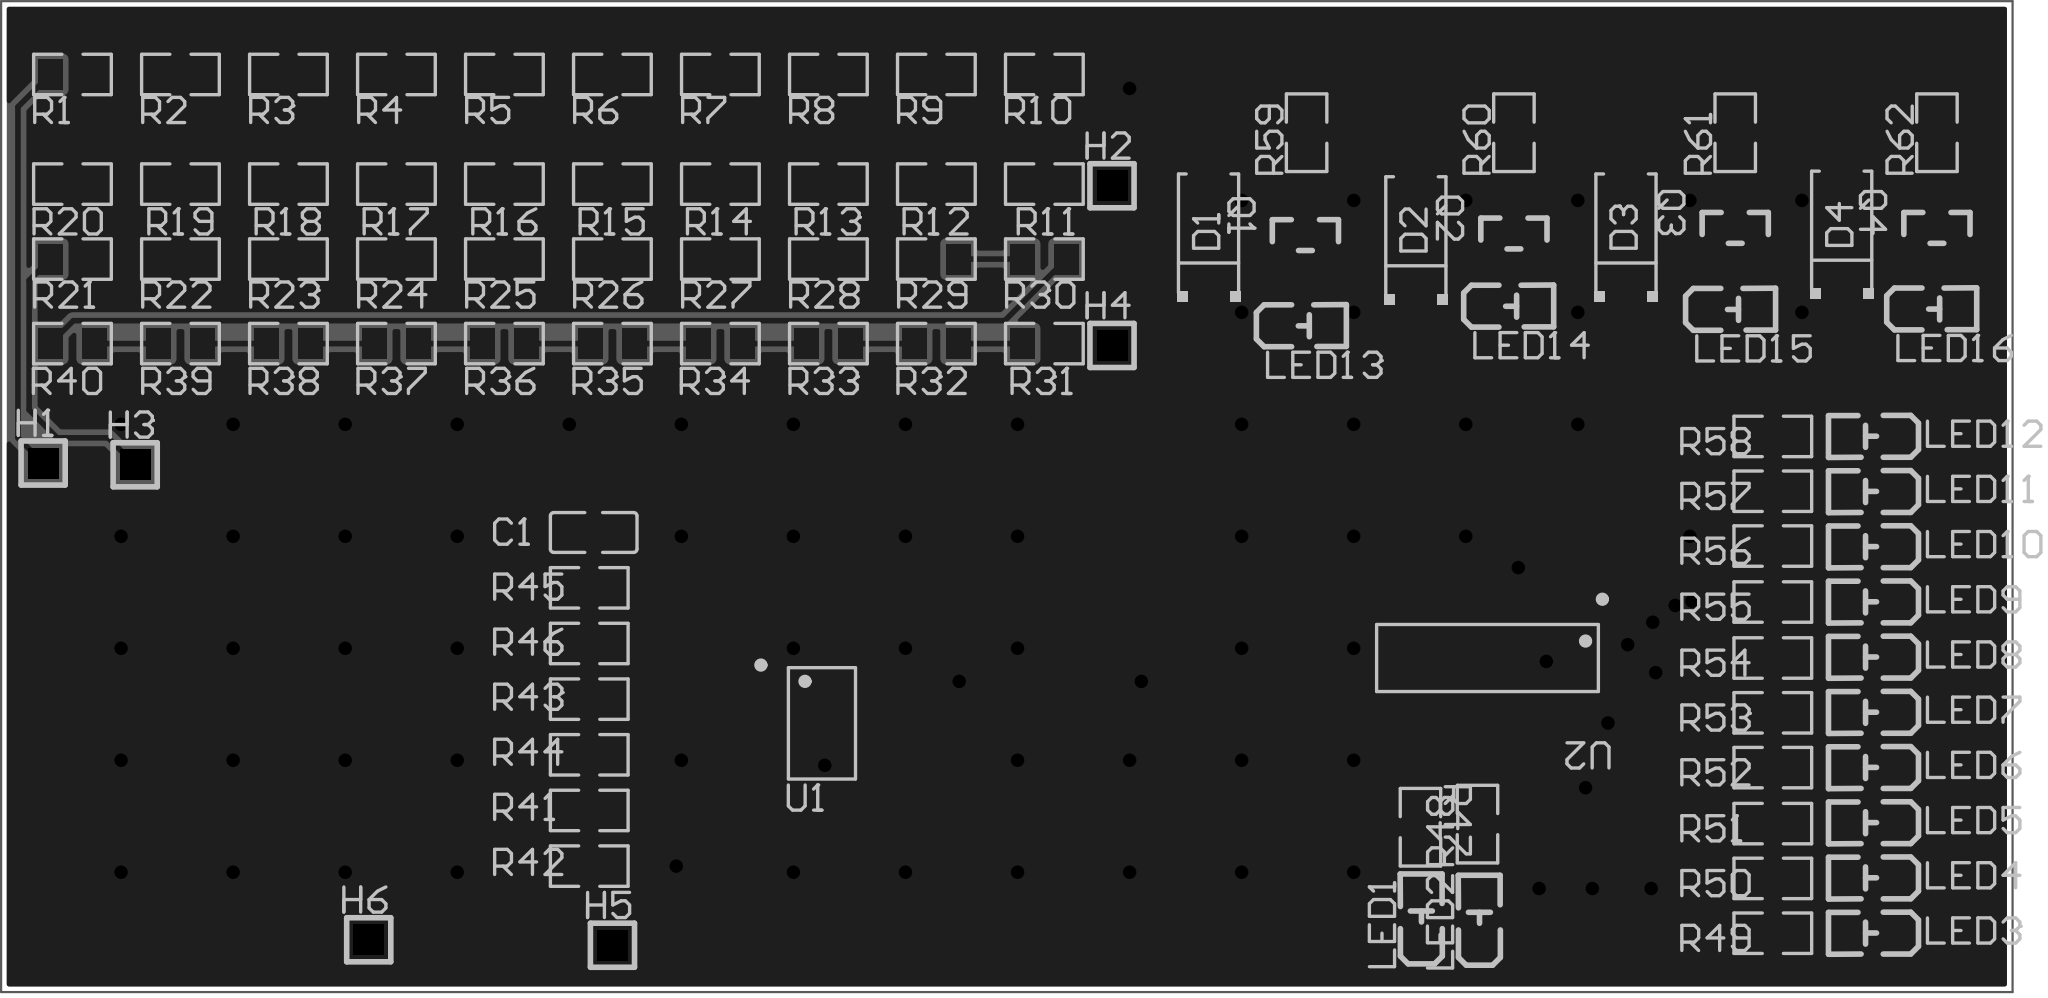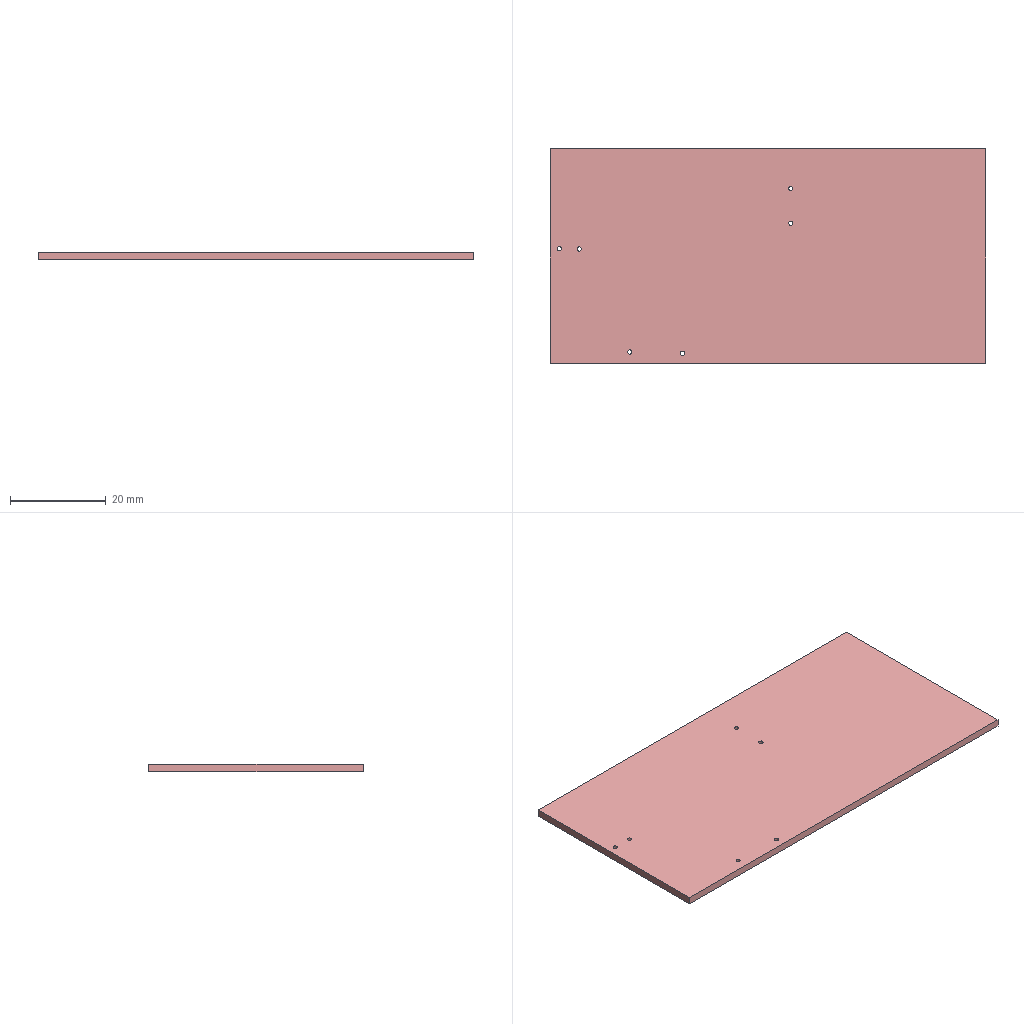Circuit board layout | Altium Designer | box 91.2 x 45 x 1.6 mm
Layer stack:
# Altium Designer layer stack of  (unit mm; dielectric type: 0 none, 1 core, 2 prepreg, 3 surface material)
index,name,kind,layer,copper_thickness_mm,dielectric_type,dielectric_thickness_mm,dielectric_material,dielectric_constant
0,Top Paste Mask Layer,other,,,,,,
1,Top Silkscreen Layer,other,,,,,,
2,Top Solder Mask Layer,dielectric,,,3,0.01,,3.3
3,Top Layer,copper,Top Layer,0.035,,,,
4,Dielectric1,dielectric,,,3,1.51,FR4,4.5
5,Bottom Layer,copper,Bottom Layer,0.035,,,,
6,Bottom Solder Mask Layer,dielectric,,,3,0.01,,3.3
7,Bottom Silkscreen Layer,other,,,,,,
8,Bottom Paste Mask Layer,other,,,,,,
# drill layer pairs: low layer,high layer
drill_pair,Top Layer,Bottom Layer
Part placement:
Designator,Comment,Layer,Footprint,Center-X(mm),Center-Y(mm),Rotation
C1,100nF,TopLayer,C0805,107.509,102.259,0
D1,,TopLayer,SMA_1N4007,135.382,115.824,90
D2,,TopLayer,SMA_1N4007,144.78,115.697,90
D3,,TopLayer,SMA_1N4007,154.305,115.824,90
D4,,TopLayer,SMA_1N4007,164.084,115.951,90
LED1,,TopLayer,LED_0805,145.029,84.786,90
LED2,,TopLayer,LED_0805,147.661,84.727,90
LED3,,TopLayer,LED_0805,165.466,84.082,180
LED4,,TopLayer,LED_0805,165.466,86.586,180
LED5,,TopLayer,LED_0805,165.466,89.091,180
LED6,,TopLayer,LED_0805,165.466,91.595,180
LED7,,TopLayer,LED_0805,165.466,94.1,180
LED8,,TopLayer,LED_0805,165.466,96.604,180
LED9,,TopLayer,LED_0805,165.466,99.108,180
LED10,,TopLayer,LED_0805,165.466,101.613,180
LED11,,TopLayer,LED_0805,165.466,104.117,180
LED12,,TopLayer,LED_0805,165.466,106.622,180
LED13,,TopLayer,LED_0805,139.65,111.638,0
LED14,,TopLayer,LED_0805,149.048,112.527,0
LED15,,TopLayer,LED_0805,159.107,112.382,0
LED16,,TopLayer,LED_0805,168.225,112.4,0
Q1,,TopLayer,S8050_SOT-23,139.773,115.751,270
Q2,,TopLayer,S8050_SOT-23,149.225,115.824,270
Q3,,TopLayer,S8050_SOT-23,159.258,116.078,270
Q4,,TopLayer,S8050_SOT-23,168.402,116.078,270
R1,10K,TopLayer,R0805,83.879,123.039,0
R2,10K,TopLayer,R0805,88.775,123.039,0
R3,10K,TopLayer,R0805,93.67,123.039,0
R4,10K,TopLayer,R0805,98.566,123.039,0
R5,10K,TopLayer,R0805,103.461,123.039,0
R6,10K,TopLayer,R0805,108.357,123.039,0
R7,10K,TopLayer,R0805,113.252,123.039,0
R8,10K,TopLayer,R0805,118.148,123.039,0
R9,10K,TopLayer,R0805,123.043,123.039,0
R10,10K,TopLayer,R0805,127.939,123.039,0
R11,10K,TopLayer,R0805,127.939,118.066,180
R12,10K,TopLayer,R0805,123.043,118.066,180
R13,10K,TopLayer,R0805,118.148,118.066,180
R14,10K,TopLayer,R0805,113.252,118.066,180
R15,10K,TopLayer,R0805,108.357,118.066,180
R16,10K,TopLayer,R0805,103.461,118.066,180
R17,10K,TopLayer,R0805,98.566,118.066,180
R18,10K,TopLayer,R0805,93.67,118.066,180
R19,10K,TopLayer,R0805,88.775,118.066,180
R20,10K,TopLayer,R0805,83.879,118.066,180
R21,15K,TopLayer,R0805,83.879,114.663,0
R22,15K,TopLayer,R0805,88.775,114.663,0
R23,15K,TopLayer,R0805,93.67,114.663,0
R24,15K,TopLayer,R0805,98.566,114.663,0
R25,15K,TopLayer,R0805,103.461,114.663,0
R26,15K,TopLayer,R0805,108.357,114.663,0
R27,15K,TopLayer,R0805,113.252,114.663,0
R28,15K,TopLayer,R0805,118.148,114.663,0
R29,15K,TopLayer,R0805,123.043,114.663,0
R30,15K,TopLayer,R0805,127.939,114.663,0
R31,15K,TopLayer,R0805,127.939,110.828,180
R32,15K,TopLayer,R0805,123.043,110.828,180
R33,15K,TopLayer,R0805,118.148,110.828,180
R34,15K,TopLayer,R0805,113.252,110.828,180
R35,15K,TopLayer,R0805,108.357,110.828,180
R36,15K,TopLayer,R0805,103.461,110.828,180
R37,15K,TopLayer,R0805,98.566,110.828,180
R38,15K,TopLayer,R0805,93.67,110.828,180
R39,15K,TopLayer,R0805,88.775,110.828,180
R40,15K,TopLayer,R0805,83.879,110.828,180
R41,10K,TopLayer,R0805,107.306,89.647,0
R42,10K,TopLayer,R0805,107.306,87.122,180
R43,10K,TopLayer,R0805,107.306,94.697,0
R44,10K,TopLayer,R0805,107.306,92.172,180
R45,10K,TopLayer,R0805,107.306,99.747,0
R46,10K,TopLayer,R0805,107.306,97.222,180
R47,1K,TopLayer,R0805,144.989,88.886,270
R48,1K,TopLayer,R0805,147.574,89.027,90
R49,10K,TopLayer,R0805,160.962,84.077,0
R50,10K,TopLayer,R0805,160.962,86.564,0
R51,10K,TopLayer,R0805,160.962,89.05,0
R52,10K,TopLayer,R0805,160.962,91.59,0
R53,10K,TopLayer,R0805,160.962,94.077,0
R54,10K,TopLayer,R0805,160.962,96.564,0
R55,10K,TopLayer,R0805,160.962,99.103,0
R56,10K,TopLayer,R0805,160.962,101.644,0
R57,10K,TopLayer,R0805,160.962,104.13,0
R58,10K,TopLayer,R0805,160.962,106.617,0
R59,1K,TopLayer,R0805,139.827,120.396,90
R60,1K,TopLayer,R0805,149.225,120.396,90
R61,1K,TopLayer,R0805,159.258,120.396,90
R62,1K,TopLayer,R0805,168.402,120.396,90
U1,NE555,TopLayer,SOP-8_L5.0-W4.0-P1.27-LS6.0-BL,117.856,93.599,270
U2,CD4017BM96G4,TopLayer,SOIC-16_L9.9-W3.9-P1.27-LS6.0-BL,148.028,96.564,180
H1,,TopLayer,HDR-TH_1P-V-M_XKB_X4611WV-01I-C28D40,82.55,105.41,0
H2,,TopLayer,HDR-TH_1P-V-M_XKB_X4611WV-01I-C28D40,131.006,117.99,0
H3,,TopLayer,HDR-TH_1P-V-M_XKB_X4611WV-01I-C28D40,86.722,105.329,0
H4,,TopLayer,HDR-TH_1P-V-M_XKB_X4611WV-01I-C28D40,131.006,110.743,0
H5,,TopLayer,HDR-TH_1P-V-M_XKB_X4611WV-01I-C28D40,108.359,83.532,0
H6,,TopLayer,HDR-TH_1P-V-M_XKB_X4611WV-01I-C28D40,97.311,83.779,0
Pad and via stacks:
# Altium Designer via and pad stacks of  (unit mm). Each distinct definition once, with the count of objects using it.
# via: kind,start_layer,end_layer,hole_mm,diameter_mm,mode(0 simple;1 top-mid-bottom;2 full stack),diameter_per_layer,count,example_net
# pad: kind,layer,hole_mm,hole_type(0 round;1 square;2 slot),plating,top_size,top_shape(1 round;2 rect;3 octagon;9 rounded rect),mid_size,bottom_size,mode,footprint,size_per_layer,count,example
pad,Top Layer,0,0,plated,1.41x1.35,2,1.41x1.35,1.41x1.35,0,C0805,,2,C1.2
pad,Top Layer,0,0,plated,2.046x1.62,2,2.046x1.62,2.046x1.62,0,SMA_1N4007,,8,D1.2
pad,Top Layer,0,0,plated,1x1.25,2,1x1.25,1x1.25,0,LED_0805,,32,LED1.2
pad,Top Layer,0,0,plated,1x0.8,2,1x0.8,1x0.8,0,S8050_SOT-23,,12,Q1.2
pad,Top Layer,0,0,plated,1.133x1.377,2,1.133x1.377,1.133x1.377,0,R0805,,124,R1.2
pad,Top Layer,0,0,plated,0.574x2.035,1,0.574x2.035,0.574x2.035,0,SOP-8_L5.0-W4.0-P1.27-LS6.0-BL,,8,U1.1
pad,Top Layer,0,0,plated,0.602x1.971,1,0.602x1.971,0.602x1.971,0,SOIC-16_L9.9-W3.9-P1.27-LS6.0-BL,,16,U2.1
pad,Multi-Layer,0.9,0,plated,1.4x1.4,2,1.4x1.4,1.4x1.4,0,HDR-TH_1P-V-M_XKB_X4611WV-01I-C28D40,,6,H1.1
via,Top Layer,Bottom Layer,0.3048,0.61,0,,80,$1N74
Copper pours:
name,layer,net,type(0 solid;1 hatched;2 none)
Top Layer-GND,Top Layer,GND,0
Bottom Layer-GND,Bottom Layer,GND,0
Design rules, without the lines most boards share:
# Altium Designer design rules of  (exported by Altium Designer, unit mm)
# columns: name | kind | enabled | priority | scope1 | scope2 | descriptor | typed fields (field=value)
creepage | 65 | enabled | 1 | All | All | Creepage Distance Constraint =(0mil) (All),(All) |
copperRegion | 20 | enabled | 1 | (InNet('GND') OR InNet('$1N69')) | All | Polygon Connect Rule(Relief Connect )(Conductor Width=10mil) (Relief Angle=90 Angle) (Entries=4) (Air Gap Width=10mil) ((InNet('GND') OR InNet('$1N69'))),(All) | connect_style(0=relief,1=direct,2=none)=0 relief_conductor_width=0.254 relief_entries=4